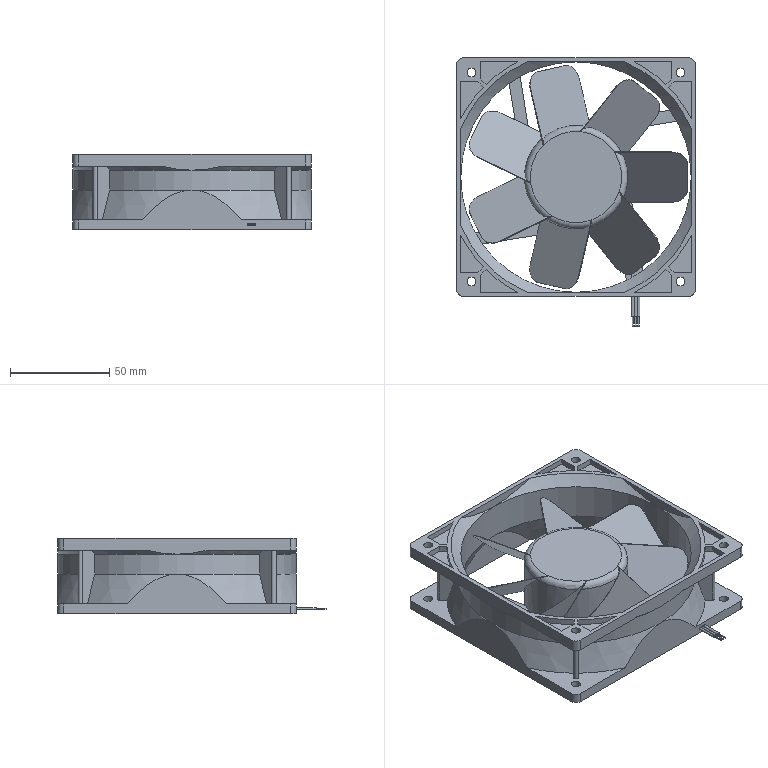Part | STEP file | E-1238D24-SRF | 1 solid | 259 faces | box 120 x 135 x 38 mm | volume 131413 mm3 | plane 162 | cylinder 66 | cone 24 | torus 7 | commonest cylinder face diameters 130 x19 16 x14 4.5 x8 6 x8 2.5 x4 120 x4